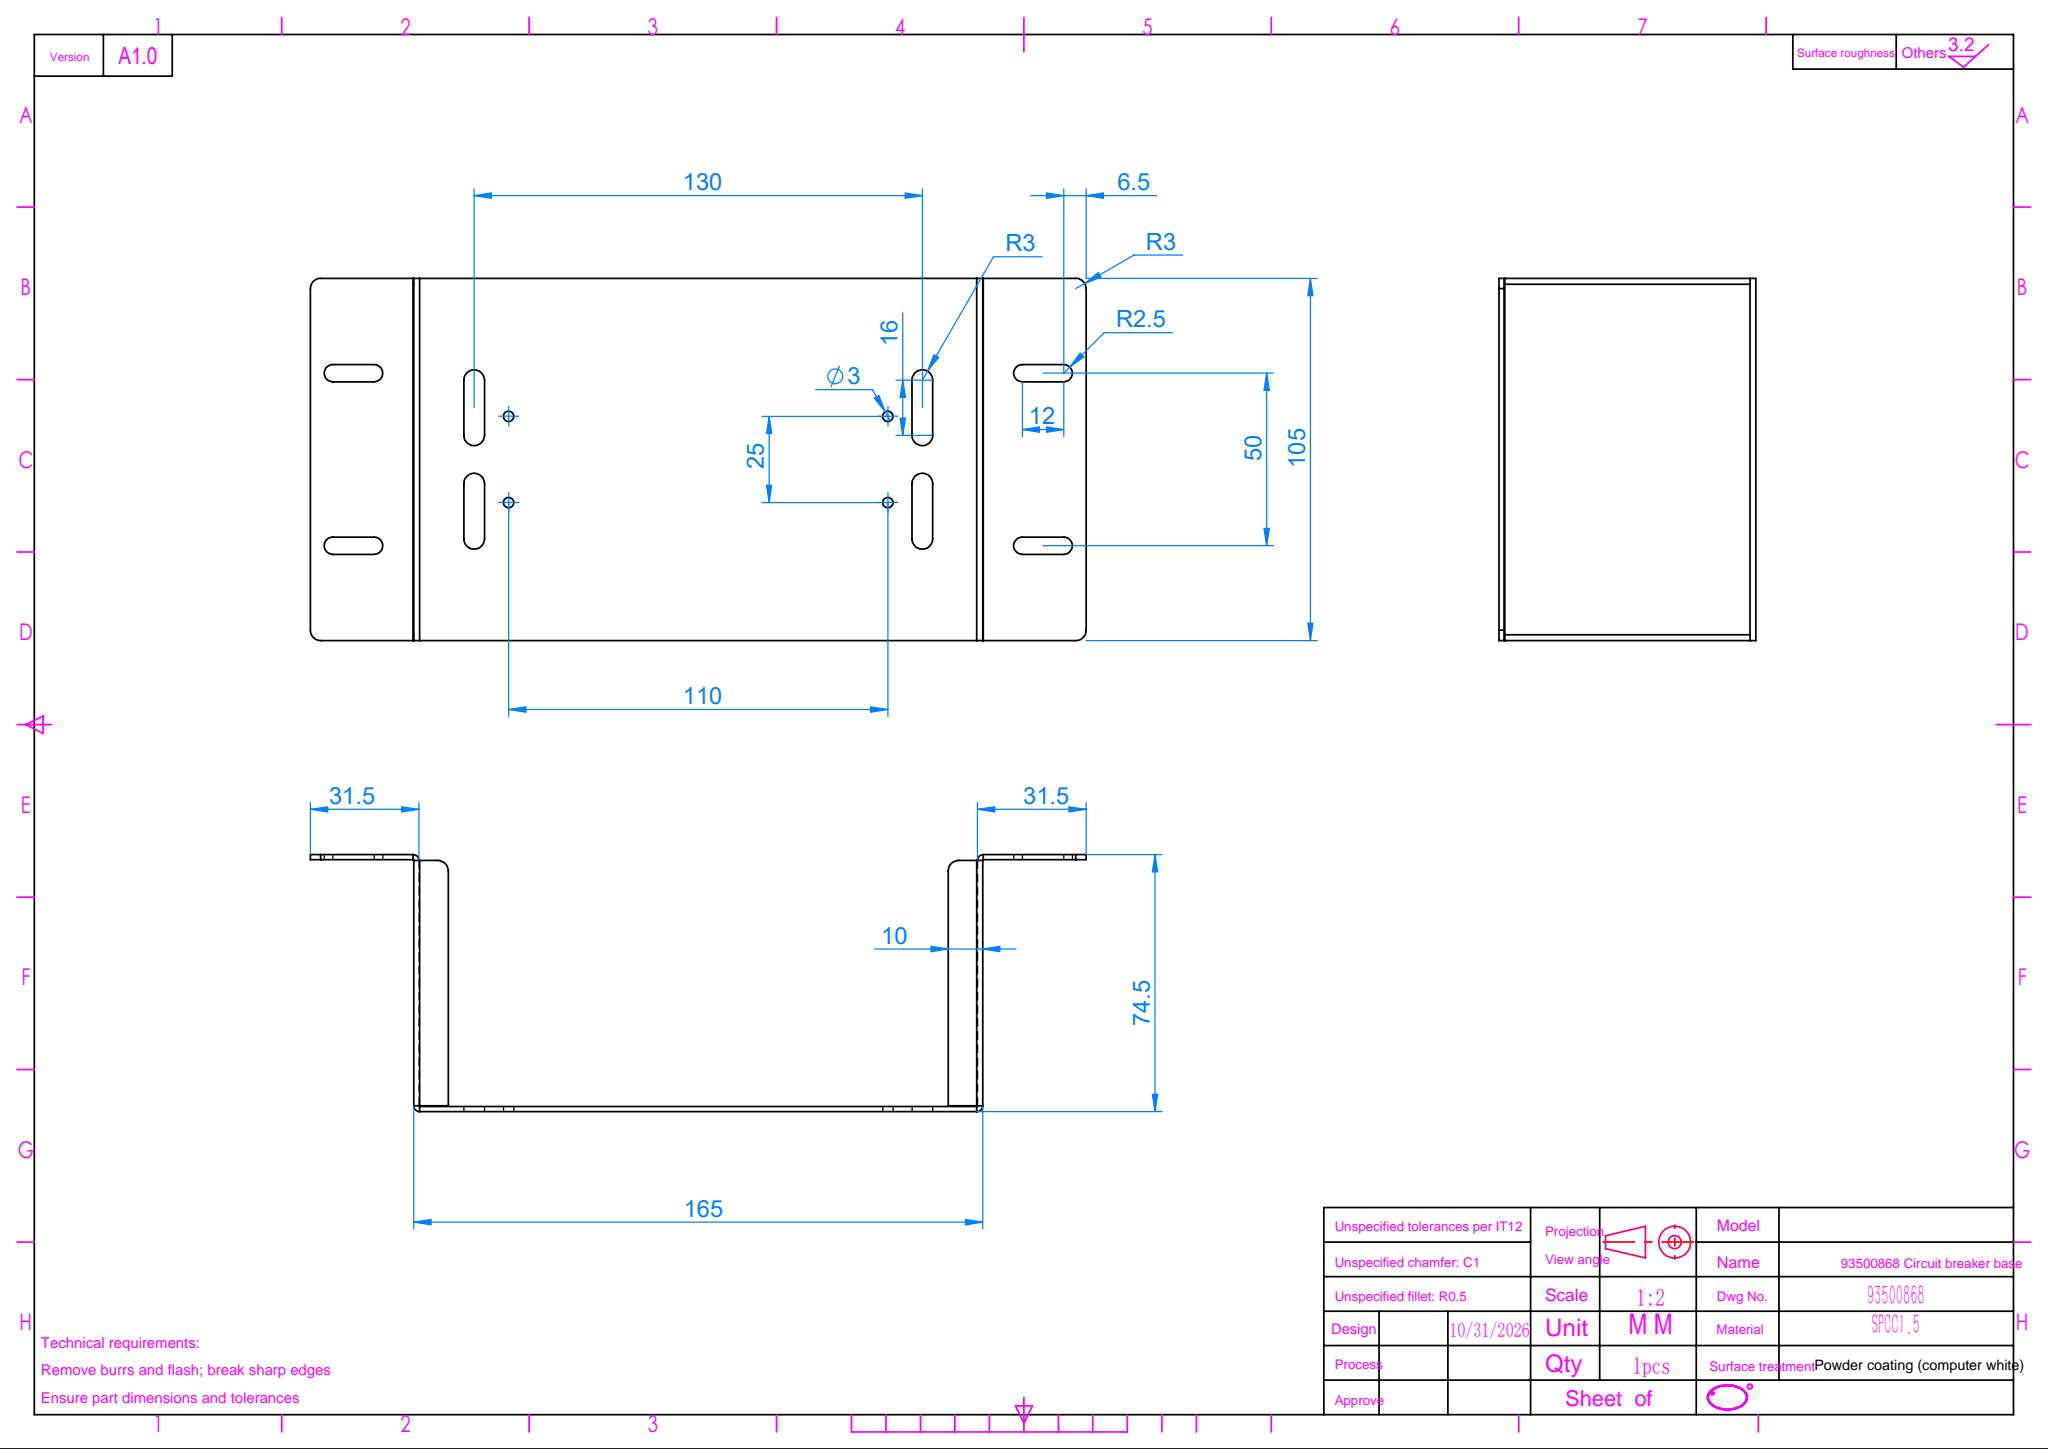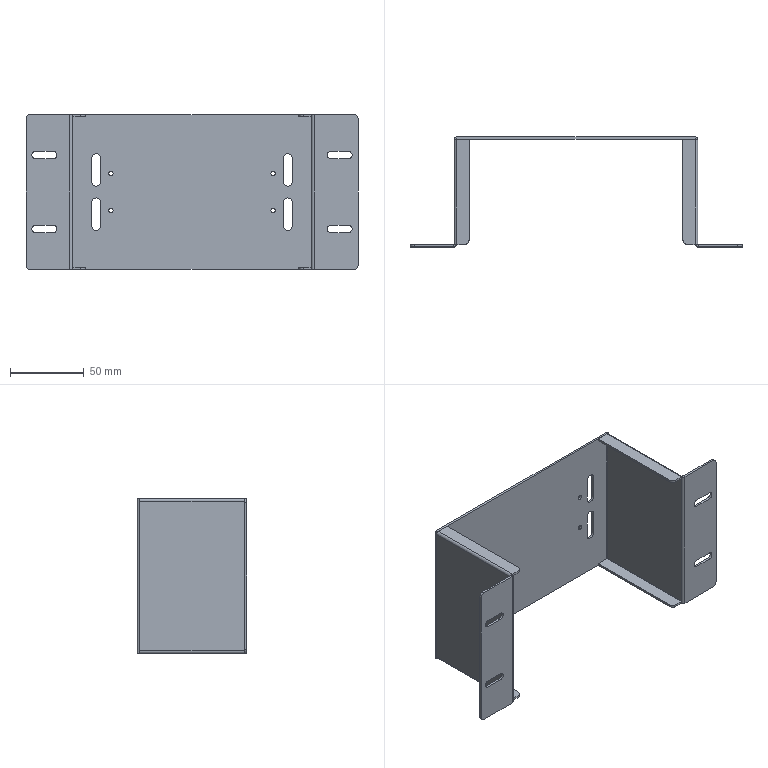Part | SolidWorks | features ICE 2, EdgeFlange 1, Fillet 1, FlatPattern 1, SMBaseFlange 1, SheetMetal 1 | 1 solid | 134 faces | box 225 x 74.5 x 105 mm | volume 60339 mm3 | plane 78 | cylinder 56 | commonest cylinder face diameters 6 x20 5 x12 0.4 x8 3 x8 3.4 x8